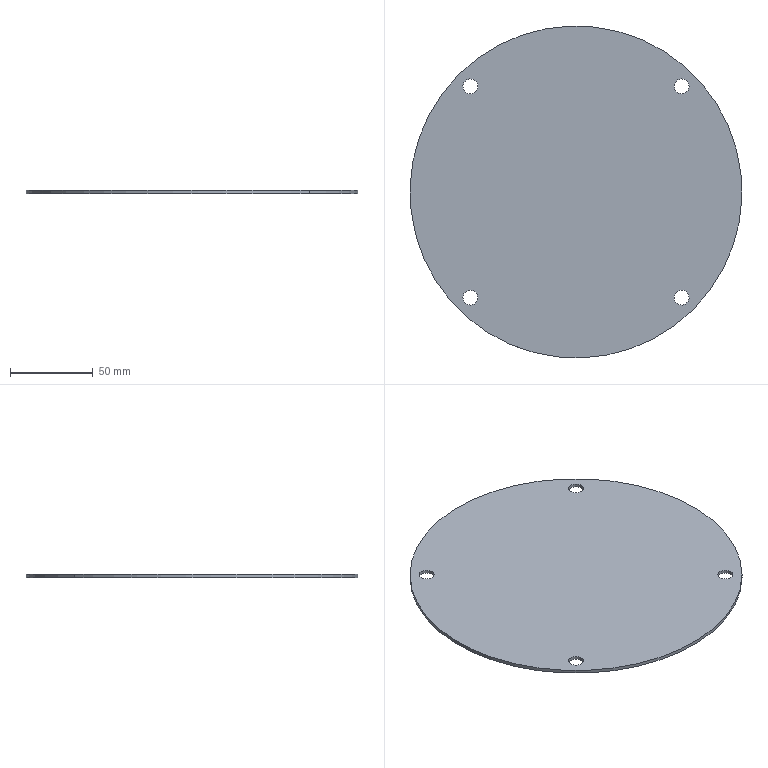Part | NX | features solid 2 | 1 solid | 12 faces | box 200 x 200 x 2 mm | volume 62323 mm3 | cylinder 10 | plane 2 | commonest cylinder face diameters 9 x8 200 x2
STEP:
#1=CARTESIAN_POINT('',(60.458,-1148.458,1456.));
#2=VERTEX_POINT('',#1);
#3=CARTESIAN_POINT('',(60.458,-1148.458,1458.));
#4=VERTEX_POINT('',#3);
#5=CARTESIAN_POINT('',(60.458,-1148.458,1175.15));
#6=DIRECTION('',(0.,0.,1.));
#7=VECTOR('',#6,1000.);
#8=LINE('',#5,#7);
#9=EDGE_CURVE('',#2,#4,#8,.T.);
#10=ORIENTED_EDGE('',*,*,#9,.F.);
#11=CARTESIAN_POINT('',(66.822,-1154.822,1456.));
#12=VERTEX_POINT('',#11);
#13=CARTESIAN_POINT('',(63.64,-1151.64,1456.));
#14=DIRECTION('',(0.,0.,-1.));
#15=DIRECTION('',(-0.7071,0.7071,0.));
#16=AXIS2_PLACEMENT_3D('',#13,#14,#15);
#17=CIRCLE('',#16,4.5);
#18=EDGE_CURVE('',#2,#12,#17,.T.);
#19=ORIENTED_EDGE('',*,*,#18,.T.);
#20=CARTESIAN_POINT('',(66.822,-1154.822,1458.));
#21=VERTEX_POINT('',#20);
#22=CARTESIAN_POINT('',(66.822,-1154.822,1175.15));
#23=DIRECTION('',(0.,0.,1.));
#24=VECTOR('',#23,1000.);
#25=LINE('',#22,#24);
#26=EDGE_CURVE('',#21,#12,#25,.F.);
#27=ORIENTED_EDGE('',*,*,#26,.F.);
#28=CARTESIAN_POINT('',(63.64,-1151.64,1458.));
#29=DIRECTION('',(0.,0.,1.));
#30=DIRECTION('',(-0.7071,0.7071,0.));
#31=AXIS2_PLACEMENT_3D('',#28,#29,#30);
#32=CIRCLE('',#31,4.5);
#33=EDGE_CURVE('',#21,#4,#32,.T.);
#34=ORIENTED_EDGE('',*,*,#33,.T.);
#35=EDGE_LOOP('',(#10,#19,#27,#34));
#36=FACE_BOUND('',#35,.T.);
#37=CARTESIAN_POINT('',(63.64,-1151.64,1175.15));
#38=DIRECTION('',(0.,0.,1.));
#39=DIRECTION('',(0.7071,-0.7071,0.));
#40=AXIS2_PLACEMENT_3D('',#37,#38,#39);
#41=CYLINDRICAL_SURFACE('',#40,4.5);
#42=ADVANCED_FACE('',(#36),#41,.F.);
#43=CARTESIAN_POINT('',(60.458,-1021.178,1456.));
#44=VERTEX_POINT('',#43);
#45=CARTESIAN_POINT('',(60.458,-1021.178,1458.));
#46=VERTEX_POINT('',#45);
#47=CARTESIAN_POINT('',(60.458,-1021.178,1175.15));
#48=DIRECTION('',(0.,0.,1.));
#49=VECTOR('',#48,1000.);
#50=LINE('',#47,#49);
#51=EDGE_CURVE('',#44,#46,#50,.T.);
#52=ORIENTED_EDGE('',*,*,#51,.F.);
#53=CARTESIAN_POINT('',(66.822,-1027.542,1456.));
#54=VERTEX_POINT('',#53);
#55=CARTESIAN_POINT('',(63.64,-1024.36,1456.));
#56=DIRECTION('',(0.,0.,-1.));
#57=DIRECTION('',(-0.7071,0.7071,0.));
#58=AXIS2_PLACEMENT_3D('',#55,#56,#57);
#59=CIRCLE('',#58,4.5);
#60=EDGE_CURVE('',#44,#54,#59,.T.);
#61=ORIENTED_EDGE('',*,*,#60,.T.);
#62=CARTESIAN_POINT('',(66.822,-1027.542,1458.));
#63=VERTEX_POINT('',#62);
#64=CARTESIAN_POINT('',(66.822,-1027.542,1175.15));
#65=DIRECTION('',(0.,0.,1.));
#66=VECTOR('',#65,1000.);
#67=LINE('',#64,#66);
#68=EDGE_CURVE('',#63,#54,#67,.F.);
#69=ORIENTED_EDGE('',*,*,#68,.F.);
#70=CARTESIAN_POINT('',(63.64,-1024.36,1458.));
#71=DIRECTION('',(0.,0.,1.));
#72=DIRECTION('',(-0.7071,0.7071,0.));
#73=AXIS2_PLACEMENT_3D('',#70,#71,#72);
#74=CIRCLE('',#73,4.5);
#75=EDGE_CURVE('',#63,#46,#74,.T.);
#76=ORIENTED_EDGE('',*,*,#75,.T.);
#77=EDGE_LOOP('',(#52,#61,#69,#76));
#78=FACE_BOUND('',#77,.T.);
#79=CARTESIAN_POINT('',(63.64,-1024.36,1175.15));
#80=DIRECTION('',(0.,0.,1.));
#81=DIRECTION('',(0.7071,-0.7071,0.));
#82=AXIS2_PLACEMENT_3D('',#79,#80,#81);
#83=CYLINDRICAL_SURFACE('',#82,4.5);
#84=ADVANCED_FACE('',(#78),#83,.F.);
#85=CARTESIAN_POINT('',(-66.822,-1021.178,1456.));
#86=VERTEX_POINT('',#85);
#87=CARTESIAN_POINT('',(-66.822,-1021.178,1458.));
#88=VERTEX_POINT('',#87);
#89=CARTESIAN_POINT('',(-66.822,-1021.178,1175.15));
#90=DIRECTION('',(0.,0.,1.));
#91=VECTOR('',#90,1000.);
#92=LINE('',#89,#91);
#93=EDGE_CURVE('',#86,#88,#92,.T.);
#94=ORIENTED_EDGE('',*,*,#93,.F.);
#95=CARTESIAN_POINT('',(-60.458,-1027.542,1456.));
#96=VERTEX_POINT('',#95);
#97=CARTESIAN_POINT('',(-63.64,-1024.36,1456.));
#98=DIRECTION('',(0.,0.,-1.));
#99=DIRECTION('',(-0.7071,0.7071,0.));
#100=AXIS2_PLACEMENT_3D('',#97,#98,#99);
#101=CIRCLE('',#100,4.5);
#102=EDGE_CURVE('',#86,#96,#101,.T.);
#103=ORIENTED_EDGE('',*,*,#102,.T.);
#104=CARTESIAN_POINT('',(-60.458,-1027.542,1458.));
#105=VERTEX_POINT('',#104);
#106=CARTESIAN_POINT('',(-60.458,-1027.542,1175.15));
#107=DIRECTION('',(0.,0.,1.));
#108=VECTOR('',#107,1000.);
#109=LINE('',#106,#108);
#110=EDGE_CURVE('',#105,#96,#109,.F.);
#111=ORIENTED_EDGE('',*,*,#110,.F.);
#112=CARTESIAN_POINT('',(-63.64,-1024.36,1458.));
#113=DIRECTION('',(0.,0.,1.));
#114=DIRECTION('',(-0.7071,0.7071,0.));
#115=AXIS2_PLACEMENT_3D('',#112,#113,#114);
#116=CIRCLE('',#115,4.5);
#117=EDGE_CURVE('',#105,#88,#116,.T.);
#118=ORIENTED_EDGE('',*,*,#117,.T.);
#119=EDGE_LOOP('',(#94,#103,#111,#118));
#120=FACE_BOUND('',#119,.T.);
#121=CARTESIAN_POINT('',(-63.64,-1024.36,1175.15));
#122=DIRECTION('',(0.,0.,1.));
#123=DIRECTION('',(0.7071,-0.7071,0.));
#124=AXIS2_PLACEMENT_3D('',#121,#122,#123);
#125=CYLINDRICAL_SURFACE('',#124,4.5);
#126=ADVANCED_FACE('',(#120),#125,.F.);
#127=CARTESIAN_POINT('',(-66.822,-1148.458,1456.));
#128=VERTEX_POINT('',#127);
#129=CARTESIAN_POINT('',(-66.822,-1148.458,1458.));
#130=VERTEX_POINT('',#129);
#131=CARTESIAN_POINT('',(-66.822,-1148.458,1175.15));
#132=DIRECTION('',(0.,0.,1.));
#133=VECTOR('',#132,1000.);
#134=LINE('',#131,#133);
#135=EDGE_CURVE('',#128,#130,#134,.T.);
#136=ORIENTED_EDGE('',*,*,#135,.F.);
#137=CARTESIAN_POINT('',(-60.458,-1154.822,1456.));
#138=VERTEX_POINT('',#137);
#139=CARTESIAN_POINT('',(-63.64,-1151.64,1456.));
#140=DIRECTION('',(0.,0.,-1.));
#141=DIRECTION('',(-0.7071,0.7071,0.));
#142=AXIS2_PLACEMENT_3D('',#139,#140,#141);
#143=CIRCLE('',#142,4.5);
#144=EDGE_CURVE('',#128,#138,#143,.T.);
#145=ORIENTED_EDGE('',*,*,#144,.T.);
#146=CARTESIAN_POINT('',(-60.458,-1154.822,1458.));
#147=VERTEX_POINT('',#146);
#148=CARTESIAN_POINT('',(-60.458,-1154.822,1175.15));
#149=DIRECTION('',(0.,0.,1.));
#150=VECTOR('',#149,1000.);
#151=LINE('',#148,#150);
#152=EDGE_CURVE('',#147,#138,#151,.F.);
#153=ORIENTED_EDGE('',*,*,#152,.F.);
#154=CARTESIAN_POINT('',(-63.64,-1151.64,1458.));
#155=DIRECTION('',(0.,0.,1.));
#156=DIRECTION('',(-0.7071,0.7071,0.));
#157=AXIS2_PLACEMENT_3D('',#154,#155,#156);
#158=CIRCLE('',#157,4.5);
#159=EDGE_CURVE('',#147,#130,#158,.T.);
#160=ORIENTED_EDGE('',*,*,#159,.T.);
#161=EDGE_LOOP('',(#136,#145,#153,#160));
#162=FACE_BOUND('',#161,.T.);
#163=CARTESIAN_POINT('',(-63.64,-1151.64,1175.15));
#164=DIRECTION('',(0.,0.,1.));
#165=DIRECTION('',(0.7071,-0.7071,0.));
#166=AXIS2_PLACEMENT_3D('',#163,#164,#165);
#167=CYLINDRICAL_SURFACE('',#166,4.5);
#168=ADVANCED_FACE('',(#162),#167,.F.);
#169=ORIENTED_EDGE('',*,*,#159,.F.);
#170=CARTESIAN_POINT('',(-63.64,-1151.64,1458.));
#171=DIRECTION('',(0.,0.,1.));
#172=DIRECTION('',(-0.7071,0.7071,0.));
#173=AXIS2_PLACEMENT_3D('',#170,#171,#172);
#174=CIRCLE('',#173,4.5);
#175=EDGE_CURVE('',#130,#147,#174,.T.);
#176=ORIENTED_EDGE('',*,*,#175,.F.);
#177=EDGE_LOOP('',(#169,#176));
#178=FACE_BOUND('',#177,.T.);
#179=ORIENTED_EDGE('',*,*,#117,.F.);
#180=CARTESIAN_POINT('',(-63.64,-1024.36,1458.));
#181=DIRECTION('',(0.,0.,1.));
#182=DIRECTION('',(-0.7071,0.7071,0.));
#183=AXIS2_PLACEMENT_3D('',#180,#181,#182);
#184=CIRCLE('',#183,4.5);
#185=EDGE_CURVE('',#88,#105,#184,.T.);
#186=ORIENTED_EDGE('',*,*,#185,.F.);
#187=EDGE_LOOP('',(#179,#186));
#188=FACE_BOUND('',#187,.T.);
#189=ORIENTED_EDGE('',*,*,#75,.F.);
#190=CARTESIAN_POINT('',(63.64,-1024.36,1458.));
#191=DIRECTION('',(0.,0.,1.));
#192=DIRECTION('',(-0.7071,0.7071,0.));
#193=AXIS2_PLACEMENT_3D('',#190,#191,#192);
#194=CIRCLE('',#193,4.5);
#195=EDGE_CURVE('',#46,#63,#194,.T.);
#196=ORIENTED_EDGE('',*,*,#195,.F.);
#197=EDGE_LOOP('',(#189,#196));
#198=FACE_BOUND('',#197,.T.);
#199=ORIENTED_EDGE('',*,*,#33,.F.);
#200=CARTESIAN_POINT('',(63.64,-1151.64,1458.));
#201=DIRECTION('',(0.,0.,1.));
#202=DIRECTION('',(-0.7071,0.7071,0.));
#203=AXIS2_PLACEMENT_3D('',#200,#201,#202);
#204=CIRCLE('',#203,4.5);
#205=EDGE_CURVE('',#4,#21,#204,.T.);
#206=ORIENTED_EDGE('',*,*,#205,.F.);
#207=EDGE_LOOP('',(#199,#206));
#208=FACE_BOUND('',#207,.T.);
#209=CARTESIAN_POINT('',(70.711,-1158.711,1458.));
#210=VERTEX_POINT('',#209);
#211=CARTESIAN_POINT('',(-70.711,-1017.289,1458.));
#212=VERTEX_POINT('',#211);
#213=CARTESIAN_POINT('',(0.,-1088.,1458.));
#214=DIRECTION('',(0.,0.,-1.));
#215=DIRECTION('',(0.7071,-0.7071,0.));
#216=AXIS2_PLACEMENT_3D('',#213,#214,#215);
#217=CIRCLE('',#216,100.);
#218=EDGE_CURVE('',#210,#212,#217,.T.);
#219=ORIENTED_EDGE('',*,*,#218,.F.);
#220=CARTESIAN_POINT('',(0.,-1088.,1458.));
#221=DIRECTION('',(0.,0.,-1.));
#222=DIRECTION('',(0.7071,-0.7071,0.));
#223=AXIS2_PLACEMENT_3D('',#220,#221,#222);
#224=CIRCLE('',#223,100.);
#225=EDGE_CURVE('',#212,#210,#224,.T.);
#226=ORIENTED_EDGE('',*,*,#225,.F.);
#227=EDGE_LOOP('',(#219,#226));
#228=FACE_BOUND('',#227,.T.);
#229=CARTESIAN_POINT('',(0.,-1088.,1458.));
#230=DIRECTION('',(0.,0.,-1.));
#231=DIRECTION('',(0.,-1.,0.));
#232=AXIS2_PLACEMENT_3D('',#229,#230,#231);
#233=PLANE('',#232);
#234=ADVANCED_FACE('',(#178,#188,#198,#208,#228),#233,.F.);
#235=CARTESIAN_POINT('',(-63.64,-1151.64,1456.));
#236=DIRECTION('',(0.,0.,-1.));
#237=DIRECTION('',(-0.7071,0.7071,0.));
#238=AXIS2_PLACEMENT_3D('',#235,#236,#237);
#239=CIRCLE('',#238,4.5);
#240=EDGE_CURVE('',#138,#128,#239,.T.);
#241=ORIENTED_EDGE('',*,*,#240,.F.);
#242=ORIENTED_EDGE('',*,*,#144,.F.);
#243=EDGE_LOOP('',(#241,#242));
#244=FACE_BOUND('',#243,.T.);
#245=CARTESIAN_POINT('',(-63.64,-1024.36,1456.));
#246=DIRECTION('',(0.,0.,-1.));
#247=DIRECTION('',(-0.7071,0.7071,0.));
#248=AXIS2_PLACEMENT_3D('',#245,#246,#247);
#249=CIRCLE('',#248,4.5);
#250=EDGE_CURVE('',#96,#86,#249,.T.);
#251=ORIENTED_EDGE('',*,*,#250,.F.);
#252=ORIENTED_EDGE('',*,*,#102,.F.);
#253=EDGE_LOOP('',(#251,#252));
#254=FACE_BOUND('',#253,.T.);
#255=CARTESIAN_POINT('',(63.64,-1024.36,1456.));
#256=DIRECTION('',(0.,0.,-1.));
#257=DIRECTION('',(-0.7071,0.7071,0.));
#258=AXIS2_PLACEMENT_3D('',#255,#256,#257);
#259=CIRCLE('',#258,4.5);
#260=EDGE_CURVE('',#54,#44,#259,.T.);
#261=ORIENTED_EDGE('',*,*,#260,.F.);
#262=ORIENTED_EDGE('',*,*,#60,.F.);
#263=EDGE_LOOP('',(#261,#262));
#264=FACE_BOUND('',#263,.T.);
#265=CARTESIAN_POINT('',(63.64,-1151.64,1456.));
#266=DIRECTION('',(0.,0.,-1.));
#267=DIRECTION('',(-0.7071,0.7071,0.));
#268=AXIS2_PLACEMENT_3D('',#265,#266,#267);
#269=CIRCLE('',#268,4.5);
#270=EDGE_CURVE('',#12,#2,#269,.T.);
#271=ORIENTED_EDGE('',*,*,#270,.F.);
#272=ORIENTED_EDGE('',*,*,#18,.F.);
#273=EDGE_LOOP('',(#271,#272));
#274=FACE_BOUND('',#273,.T.);
#275=CARTESIAN_POINT('',(70.711,-1158.711,1456.));
#276=VERTEX_POINT('',#275);
#277=CARTESIAN_POINT('',(-70.711,-1017.289,1456.));
#278=VERTEX_POINT('',#277);
#279=CARTESIAN_POINT('',(0.,-1088.,1456.));
#280=DIRECTION('',(0.,0.,-1.));
#281=DIRECTION('',(0.7071,-0.7071,0.));
#282=AXIS2_PLACEMENT_3D('',#279,#280,#281);
#283=CIRCLE('',#282,100.);
#284=EDGE_CURVE('',#276,#278,#283,.T.);
#285=ORIENTED_EDGE('',*,*,#284,.T.);
#286=CARTESIAN_POINT('',(0.,-1088.,1456.));
#287=DIRECTION('',(0.,0.,-1.));
#288=DIRECTION('',(0.7071,-0.7071,0.));
#289=AXIS2_PLACEMENT_3D('',#286,#287,#288);
#290=CIRCLE('',#289,100.);
#291=EDGE_CURVE('',#278,#276,#290,.T.);
#292=ORIENTED_EDGE('',*,*,#291,.T.);
#293=EDGE_LOOP('',(#285,#292));
#294=FACE_BOUND('',#293,.T.);
#295=CARTESIAN_POINT('',(0.,-1088.,1456.));
#296=DIRECTION('',(0.,0.,-1.));
#297=DIRECTION('',(0.,-1.,0.));
#298=AXIS2_PLACEMENT_3D('',#295,#296,#297);
#299=PLANE('',#298);
#300=ADVANCED_FACE('',(#244,#254,#264,#274,#294),#299,.T.);
#301=CARTESIAN_POINT('',(-70.711,-1017.289,1456.));
#302=DIRECTION('',(0.,0.,1.));
#303=VECTOR('',#302,1000.);
#304=LINE('',#301,#303);
#305=EDGE_CURVE('',#212,#278,#304,.F.);
#306=ORIENTED_EDGE('',*,*,#305,.T.);
#307=ORIENTED_EDGE('',*,*,#284,.F.);
#308=CARTESIAN_POINT('',(70.711,-1158.711,1456.));
#309=DIRECTION('',(0.,0.,1.));
#310=VECTOR('',#309,1000.);
#311=LINE('',#308,#310);
#312=EDGE_CURVE('',#276,#210,#311,.T.);
#313=ORIENTED_EDGE('',*,*,#312,.T.);
#314=ORIENTED_EDGE('',*,*,#218,.T.);
#315=EDGE_LOOP('',(#306,#307,#313,#314));
#316=FACE_BOUND('',#315,.T.);
#317=CARTESIAN_POINT('',(0.,-1088.,1456.));
#318=DIRECTION('',(0.,0.,1.));
#319=DIRECTION('',(0.7071,-0.7071,0.));
#320=AXIS2_PLACEMENT_3D('',#317,#318,#319);
#321=CYLINDRICAL_SURFACE('',#320,100.);
#322=ADVANCED_FACE('',(#316),#321,.T.);
#323=ORIENTED_EDGE('',*,*,#291,.F.);
#324=ORIENTED_EDGE('',*,*,#305,.F.);
#325=ORIENTED_EDGE('',*,*,#225,.T.);
#326=ORIENTED_EDGE('',*,*,#312,.F.);
#327=EDGE_LOOP('',(#323,#324,#325,#326));
#328=FACE_BOUND('',#327,.T.);
#329=CARTESIAN_POINT('',(0.,-1088.,1456.));
#330=DIRECTION('',(0.,0.,1.));
#331=DIRECTION('',(0.7071,-0.7071,0.));
#332=AXIS2_PLACEMENT_3D('',#329,#330,#331);
#333=CYLINDRICAL_SURFACE('',#332,100.);
#334=ADVANCED_FACE('',(#328),#333,.T.);
#335=ORIENTED_EDGE('',*,*,#240,.T.);
#336=ORIENTED_EDGE('',*,*,#135,.T.);
#337=ORIENTED_EDGE('',*,*,#175,.T.);
#338=ORIENTED_EDGE('',*,*,#152,.T.);
#339=EDGE_LOOP('',(#335,#336,#337,#338));
#340=FACE_BOUND('',#339,.T.);
#341=CARTESIAN_POINT('',(-63.64,-1151.64,1175.15));
#342=DIRECTION('',(0.,0.,1.));
#343=DIRECTION('',(0.7071,-0.7071,0.));
#344=AXIS2_PLACEMENT_3D('',#341,#342,#343);
#345=CYLINDRICAL_SURFACE('',#344,4.5);
#346=ADVANCED_FACE('',(#340),#345,.F.);
#347=ORIENTED_EDGE('',*,*,#250,.T.);
#348=ORIENTED_EDGE('',*,*,#93,.T.);
#349=ORIENTED_EDGE('',*,*,#185,.T.);
#350=ORIENTED_EDGE('',*,*,#110,.T.);
#351=EDGE_LOOP('',(#347,#348,#349,#350));
#352=FACE_BOUND('',#351,.T.);
#353=CARTESIAN_POINT('',(-63.64,-1024.36,1175.15));
#354=DIRECTION('',(0.,0.,1.));
#355=DIRECTION('',(0.7071,-0.7071,0.));
#356=AXIS2_PLACEMENT_3D('',#353,#354,#355);
#357=CYLINDRICAL_SURFACE('',#356,4.5);
#358=ADVANCED_FACE('',(#352),#357,.F.);
#359=ORIENTED_EDGE('',*,*,#260,.T.);
#360=ORIENTED_EDGE('',*,*,#51,.T.);
#361=ORIENTED_EDGE('',*,*,#195,.T.);
#362=ORIENTED_EDGE('',*,*,#68,.T.);
#363=EDGE_LOOP('',(#359,#360,#361,#362));
#364=FACE_BOUND('',#363,.T.);
#365=CARTESIAN_POINT('',(63.64,-1024.36,1175.15));
#366=DIRECTION('',(0.,0.,1.));
#367=DIRECTION('',(0.7071,-0.7071,0.));
#368=AXIS2_PLACEMENT_3D('',#365,#366,#367);
#369=CYLINDRICAL_SURFACE('',#368,4.5);
#370=ADVANCED_FACE('',(#364),#369,.F.);
#371=ORIENTED_EDGE('',*,*,#270,.T.);
#372=ORIENTED_EDGE('',*,*,#9,.T.);
#373=ORIENTED_EDGE('',*,*,#205,.T.);
#374=ORIENTED_EDGE('',*,*,#26,.T.);
#375=EDGE_LOOP('',(#371,#372,#373,#374));
#376=FACE_BOUND('',#375,.T.);
#377=CARTESIAN_POINT('',(63.64,-1151.64,1175.15));
#378=DIRECTION('',(0.,0.,1.));
#379=DIRECTION('',(0.7071,-0.7071,0.));
#380=AXIS2_PLACEMENT_3D('',#377,#378,#379);
#381=CYLINDRICAL_SURFACE('',#380,4.5);
#382=ADVANCED_FACE('',(#376),#381,.F.);
#383=CLOSED_SHELL('',(#42,#84,#126,#168,#234,#300,#322,#334,#346,#358,#370,#382));
#384=MANIFOLD_SOLID_BREP('',#383);
#385=(LENGTH_UNIT()NAMED_UNIT(*)SI_UNIT(.MILLI.,.METRE.));
#386=UNCERTAINTY_MEASURE_WITH_UNIT(LENGTH_MEASURE(0.00001),#385,'','');
#387=(NAMED_UNIT(*)PLANE_ANGLE_UNIT()SI_UNIT($,.RADIAN.));
#388=(NAMED_UNIT(*)SI_UNIT($,.STERADIAN.)SOLID_ANGLE_UNIT());
#389=(GEOMETRIC_REPRESENTATION_CONTEXT(3)GLOBAL_UNCERTAINTY_ASSIGNED_CONTEXT((#386))GLOBAL_UNIT_ASSIGNED_CONTEXT((#385,#387,#388))REPRESENTATION_CONTEXT('',''));
#390=ADVANCED_BREP_SHAPE_REPRESENTATION('',(#384),#389);